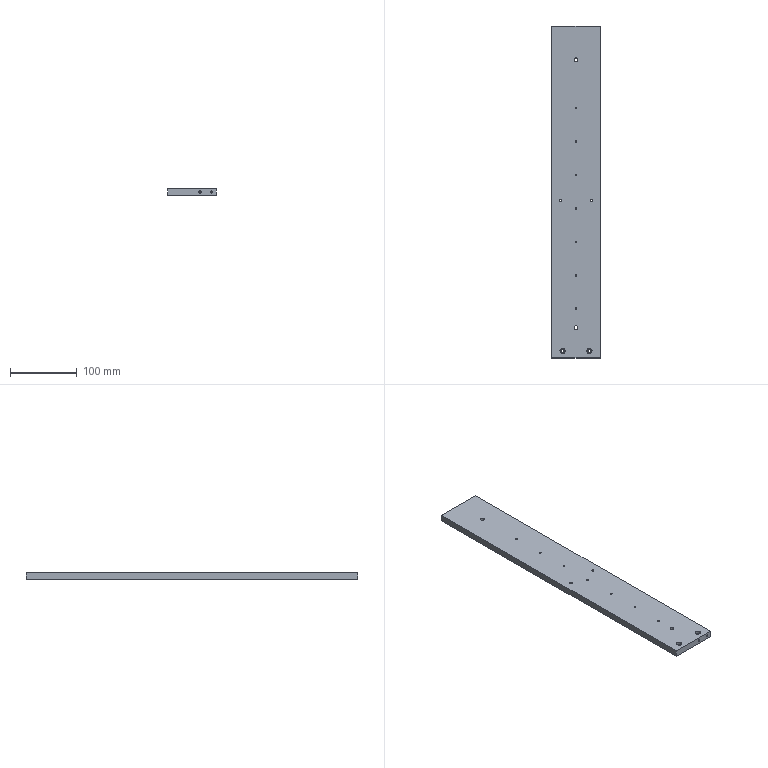Part | SolidWorks | features HoleWzd 6, Extrusion 1 | 1 solid | 52 faces | box 72 x 496 x 10 mm | volume 354695 mm3 | cylinder 38 | plane 10 | cone 4 | commonest cylinder face diameters 2.5 x14 3.3 x8 4.5 x4 5.5 x4 8 x4 10 x4